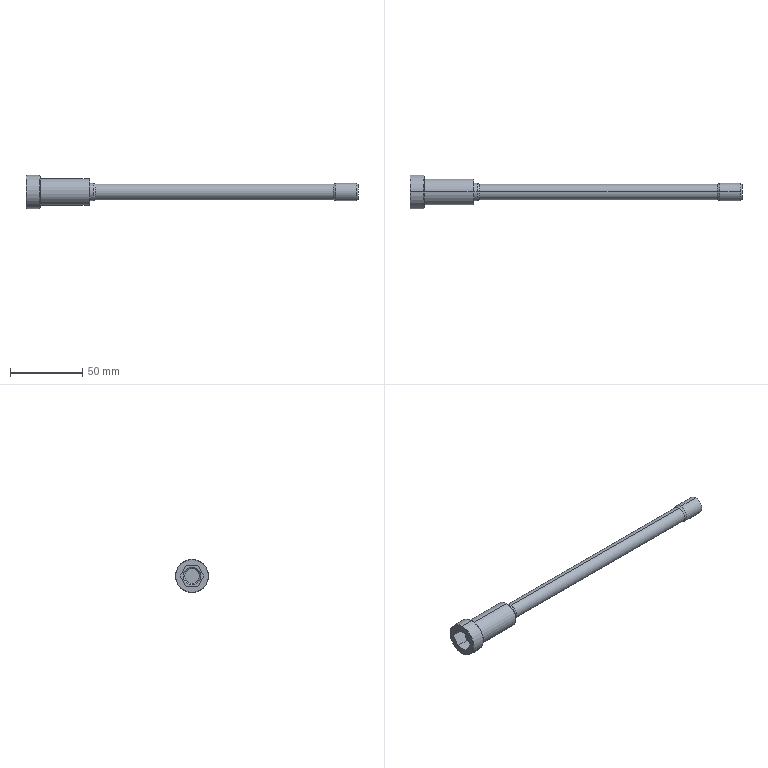Part | STEP file | SI125_100 | 1 solid | 40 faces | box 229 x 23 x 23 mm | volume 26523 mm3 | cone 16 | cylinder 12 | plane 12 | commonest cylinder face diameters 12 x4 10.106 x2 10.7 x2 18 x2 23 x2